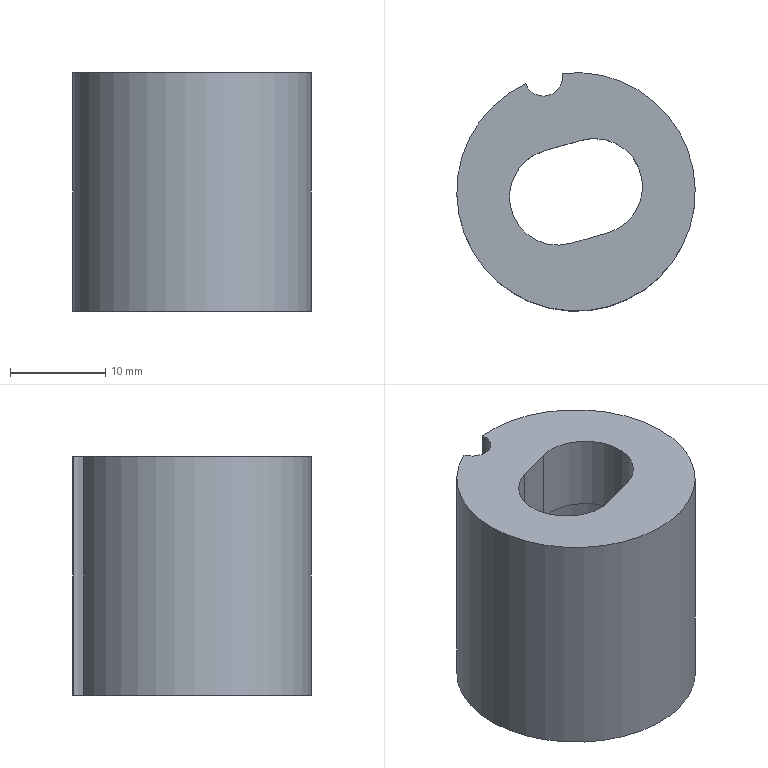Part | NX | features solid 2 | 1 solid | 10 faces | box 25 x 25 x 25 mm | volume 7477 mm3 | cylinder 5 | plane 5 | commonest cylinder face diameters 10.1 x2 4 x1 16.6 x1 25 x1
STEP:
#1=CARTESIAN_POINT('',(529.721,-368.981,-7.));
#2=VERTEX_POINT('',#1);
#3=CARTESIAN_POINT('',(529.721,-368.981,18.));
#4=VERTEX_POINT('',#3);
#5=CARTESIAN_POINT('',(529.721,-368.981,5.5));
#6=DIRECTION('',(0.,0.,1.));
#7=VECTOR('',#6,1000.);
#8=LINE('',#5,#7);
#9=EDGE_CURVE('',#2,#4,#8,.T.);
#10=ORIENTED_EDGE('',*,*,#9,.F.);
#11=CARTESIAN_POINT('',(533.558,-367.895,-7.));
#12=VERTEX_POINT('',#11);
#13=CARTESIAN_POINT('',(535.,-380.311,-7.));
#14=DIRECTION('',(0.,0.,1.));
#15=DIRECTION('',(-0.2723,0.9622,0.));
#16=AXIS2_PLACEMENT_3D('',#13,#14,#15);
#17=CIRCLE('',#16,12.5);
#18=EDGE_CURVE('',#2,#12,#17,.T.);
#19=ORIENTED_EDGE('',*,*,#18,.T.);
#20=CARTESIAN_POINT('',(533.558,-367.895,18.));
#21=VERTEX_POINT('',#20);
#22=CARTESIAN_POINT('',(533.558,-367.895,5.5));
#23=DIRECTION('',(0.,0.,1.));
#24=VECTOR('',#23,1000.);
#25=LINE('',#22,#24);
#26=EDGE_CURVE('',#21,#12,#25,.F.);
#27=ORIENTED_EDGE('',*,*,#26,.F.);
#28=CARTESIAN_POINT('',(535.,-380.311,18.));
#29=DIRECTION('',(0.,0.,1.));
#30=DIRECTION('',(-0.2723,0.9622,0.));
#31=AXIS2_PLACEMENT_3D('',#28,#29,#30);
#32=CIRCLE('',#31,12.5);
#33=EDGE_CURVE('',#4,#21,#32,.T.);
#34=ORIENTED_EDGE('',*,*,#33,.F.);
#35=EDGE_LOOP('',(#10,#19,#27,#34));
#36=FACE_BOUND('',#35,.T.);
#37=CARTESIAN_POINT('',(535.,-380.311,-7.));
#38=DIRECTION('',(0.,0.,1.));
#39=DIRECTION('',(-0.2723,0.9622,0.));
#40=AXIS2_PLACEMENT_3D('',#37,#38,#39);
#41=CYLINDRICAL_SURFACE('',#40,12.5);
#42=ADVANCED_FACE('',(#36),#41,.T.);
#43=CARTESIAN_POINT('',(532.74,-372.325,-7.));
#44=VERTEX_POINT('',#43);
#45=CARTESIAN_POINT('',(535.,-380.311,-7.));
#46=DIRECTION('',(0.,0.,1.));
#47=DIRECTION('',(-0.2723,0.9622,0.));
#48=AXIS2_PLACEMENT_3D('',#45,#46,#47);
#49=CIRCLE('',#48,8.3);
#50=EDGE_CURVE('',#44,#44,#49,.T.);
#51=ORIENTED_EDGE('',*,*,#50,.T.);
#52=EDGE_LOOP('',(#51));
#53=FACE_BOUND('',#52,.T.);
#54=ORIENTED_EDGE('',*,*,#18,.F.);
#55=CARTESIAN_POINT('',(531.596,-368.284,-7.));
#56=DIRECTION('',(0.,0.,1.));
#57=DIRECTION('',(-0.2723,0.9622,0.));
#58=AXIS2_PLACEMENT_3D('',#55,#56,#57);
#59=CIRCLE('',#58,2.);
#60=EDGE_CURVE('',#2,#12,#59,.T.);
#61=ORIENTED_EDGE('',*,*,#60,.T.);
#62=EDGE_LOOP('',(#54,#61));
#63=FACE_BOUND('',#62,.T.);
#64=CARTESIAN_POINT('',(535.,-380.311,-7.));
#65=DIRECTION('',(0.,0.,1.));
#66=DIRECTION('',(-0.2723,0.9622,0.));
#67=AXIS2_PLACEMENT_3D('',#64,#65,#66);
#68=PLANE('',#67);
#69=ADVANCED_FACE('',(#53,#63),#68,.F.);
#70=CARTESIAN_POINT('',(534.451,-385.715,18.));
#71=VERTEX_POINT('',#70);
#72=CARTESIAN_POINT('',(538.3,-384.626,18.));
#73=VERTEX_POINT('',#72);
#74=CARTESIAN_POINT('',(534.451,-385.715,18.));
#75=DIRECTION('',(0.9622,0.2723,0.));
#76=VECTOR('',#75,1000.);
#77=LINE('',#74,#76);
#78=EDGE_CURVE('',#71,#73,#77,.T.);
#79=ORIENTED_EDGE('',*,*,#78,.F.);
#80=CARTESIAN_POINT('',(531.7,-375.997,18.));
#81=VERTEX_POINT('',#80);
#82=CARTESIAN_POINT('',(533.076,-380.856,18.));
#83=DIRECTION('',(0.,0.,1.));
#84=DIRECTION('',(-0.2723,0.9622,0.));
#85=AXIS2_PLACEMENT_3D('',#82,#83,#84);
#86=CIRCLE('',#85,5.05);
#87=EDGE_CURVE('',#81,#71,#86,.T.);
#88=ORIENTED_EDGE('',*,*,#87,.F.);
#89=CARTESIAN_POINT('',(535.549,-374.908,18.));
#90=VERTEX_POINT('',#89);
#91=CARTESIAN_POINT('',(531.7,-375.997,18.));
#92=DIRECTION('',(0.9622,0.2723,0.));
#93=VECTOR('',#92,1000.);
#94=LINE('',#91,#93);
#95=EDGE_CURVE('',#81,#90,#94,.T.);
#96=ORIENTED_EDGE('',*,*,#95,.T.);
#97=CARTESIAN_POINT('',(536.924,-379.767,18.));
#98=DIRECTION('',(0.,0.,1.));
#99=DIRECTION('',(-0.2723,0.9622,0.));
#100=AXIS2_PLACEMENT_3D('',#97,#98,#99);
#101=CIRCLE('',#100,5.05);
#102=EDGE_CURVE('',#73,#90,#101,.T.);
#103=ORIENTED_EDGE('',*,*,#102,.F.);
#104=EDGE_LOOP('',(#79,#88,#96,#103));
#105=FACE_BOUND('',#104,.T.);
#106=CARTESIAN_POINT('',(531.596,-368.284,18.));
#107=DIRECTION('',(0.,0.,1.));
#108=DIRECTION('',(-0.2723,0.9622,0.));
#109=AXIS2_PLACEMENT_3D('',#106,#107,#108);
#110=CIRCLE('',#109,2.);
#111=EDGE_CURVE('',#4,#21,#110,.T.);
#112=ORIENTED_EDGE('',*,*,#111,.F.);
#113=ORIENTED_EDGE('',*,*,#33,.T.);
#114=EDGE_LOOP('',(#112,#113));
#115=FACE_BOUND('',#114,.T.);
#116=CARTESIAN_POINT('',(535.,-380.311,18.));
#117=DIRECTION('',(0.,0.,1.));
#118=DIRECTION('',(-0.2723,0.9622,0.));
#119=AXIS2_PLACEMENT_3D('',#116,#117,#118);
#120=PLANE('',#119);
#121=ADVANCED_FACE('',(#105,#115),#120,.T.);
#122=ORIENTED_EDGE('',*,*,#50,.F.);
#123=EDGE_LOOP('',(#122));
#124=FACE_BOUND('',#123,.T.);
#125=CARTESIAN_POINT('',(532.74,-372.325,10.));
#126=VERTEX_POINT('',#125);
#127=CARTESIAN_POINT('',(535.,-380.311,10.));
#128=DIRECTION('',(0.,0.,1.));
#129=DIRECTION('',(-0.2723,0.9622,0.));
#130=AXIS2_PLACEMENT_3D('',#127,#128,#129);
#131=CIRCLE('',#130,8.3);
#132=EDGE_CURVE('',#126,#126,#131,.T.);
#133=ORIENTED_EDGE('',*,*,#132,.T.);
#134=EDGE_LOOP('',(#133));
#135=FACE_BOUND('',#134,.T.);
#136=CARTESIAN_POINT('',(535.,-380.311,-7.));
#137=DIRECTION('',(0.,0.,1.));
#138=DIRECTION('',(-0.2723,0.9622,0.));
#139=AXIS2_PLACEMENT_3D('',#136,#137,#138);
#140=CYLINDRICAL_SURFACE('',#139,8.3);
#141=ADVANCED_FACE('',(#124,#135),#140,.F.);
#142=CARTESIAN_POINT('',(531.7,-375.997,10.));
#143=VERTEX_POINT('',#142);
#144=CARTESIAN_POINT('',(534.451,-385.715,10.));
#145=VERTEX_POINT('',#144);
#146=CARTESIAN_POINT('',(533.076,-380.856,10.));
#147=DIRECTION('',(0.,0.,1.));
#148=DIRECTION('',(-0.2723,0.9622,0.));
#149=AXIS2_PLACEMENT_3D('',#146,#147,#148);
#150=CIRCLE('',#149,5.05);
#151=EDGE_CURVE('',#143,#145,#150,.T.);
#152=ORIENTED_EDGE('',*,*,#151,.T.);
#153=CARTESIAN_POINT('',(538.3,-384.626,10.));
#154=VERTEX_POINT('',#153);
#155=CARTESIAN_POINT('',(536.375,-385.171,10.));
#156=DIRECTION('',(0.9622,0.2723,0.));
#157=VECTOR('',#156,1000.);
#158=LINE('',#155,#157);
#159=EDGE_CURVE('',#145,#154,#158,.T.);
#160=ORIENTED_EDGE('',*,*,#159,.T.);
#161=CARTESIAN_POINT('',(535.549,-374.908,10.));
#162=VERTEX_POINT('',#161);
#163=CARTESIAN_POINT('',(536.924,-379.767,10.));
#164=DIRECTION('',(0.,0.,1.));
#165=DIRECTION('',(-0.2723,0.9622,0.));
#166=AXIS2_PLACEMENT_3D('',#163,#164,#165);
#167=CIRCLE('',#166,5.05);
#168=EDGE_CURVE('',#154,#162,#167,.T.);
#169=ORIENTED_EDGE('',*,*,#168,.T.);
#170=CARTESIAN_POINT('',(533.625,-375.452,10.));
#171=DIRECTION('',(0.9622,0.2723,0.));
#172=VECTOR('',#171,1000.);
#173=LINE('',#170,#172);
#174=EDGE_CURVE('',#143,#162,#173,.T.);
#175=ORIENTED_EDGE('',*,*,#174,.F.);
#176=EDGE_LOOP('',(#152,#160,#169,#175));
#177=FACE_BOUND('',#176,.T.);
#178=ORIENTED_EDGE('',*,*,#132,.F.);
#179=EDGE_LOOP('',(#178));
#180=FACE_BOUND('',#179,.T.);
#181=CARTESIAN_POINT('',(535.,-380.311,10.));
#182=DIRECTION('',(0.,0.,1.));
#183=DIRECTION('',(-0.2723,0.9622,0.));
#184=AXIS2_PLACEMENT_3D('',#181,#182,#183);
#185=PLANE('',#184);
#186=ADVANCED_FACE('',(#177,#180),#185,.F.);
#187=ORIENTED_EDGE('',*,*,#9,.T.);
#188=ORIENTED_EDGE('',*,*,#111,.T.);
#189=ORIENTED_EDGE('',*,*,#26,.T.);
#190=ORIENTED_EDGE('',*,*,#60,.F.);
#191=EDGE_LOOP('',(#187,#188,#189,#190));
#192=FACE_BOUND('',#191,.T.);
#193=CARTESIAN_POINT('',(531.596,-368.284,-7.));
#194=DIRECTION('',(0.,0.,1.));
#195=DIRECTION('',(-0.2723,0.9622,0.));
#196=AXIS2_PLACEMENT_3D('',#193,#194,#195);
#197=CYLINDRICAL_SURFACE('',#196,2.);
#198=ADVANCED_FACE('',(#192),#197,.F.);
#199=CARTESIAN_POINT('',(534.451,-385.715,-7.));
#200=DIRECTION('',(0.,0.,1.));
#201=VECTOR('',#200,1000.);
#202=LINE('',#199,#201);
#203=EDGE_CURVE('',#145,#71,#202,.T.);
#204=ORIENTED_EDGE('',*,*,#203,.T.);
#205=ORIENTED_EDGE('',*,*,#78,.T.);
#206=CARTESIAN_POINT('',(538.3,-384.626,-7.));
#207=DIRECTION('',(0.,0.,1.));
#208=VECTOR('',#207,1000.);
#209=LINE('',#206,#208);
#210=EDGE_CURVE('',#154,#73,#209,.T.);
#211=ORIENTED_EDGE('',*,*,#210,.F.);
#212=ORIENTED_EDGE('',*,*,#159,.F.);
#213=EDGE_LOOP('',(#204,#205,#211,#212));
#214=FACE_BOUND('',#213,.T.);
#215=CARTESIAN_POINT('',(534.451,-385.715,-7.));
#216=DIRECTION('',(0.2723,-0.9622,0.));
#217=DIRECTION('',(0.,0.,1.));
#218=AXIS2_PLACEMENT_3D('',#215,#216,#217);
#219=PLANE('',#218);
#220=ADVANCED_FACE('',(#214),#219,.F.);
#221=ORIENTED_EDGE('',*,*,#210,.T.);
#222=ORIENTED_EDGE('',*,*,#102,.T.);
#223=CARTESIAN_POINT('',(535.549,-374.908,-7.));
#224=DIRECTION('',(0.,0.,1.));
#225=VECTOR('',#224,1000.);
#226=LINE('',#223,#225);
#227=EDGE_CURVE('',#162,#90,#226,.T.);
#228=ORIENTED_EDGE('',*,*,#227,.F.);
#229=ORIENTED_EDGE('',*,*,#168,.F.);
#230=EDGE_LOOP('',(#221,#222,#228,#229));
#231=FACE_BOUND('',#230,.T.);
#232=CARTESIAN_POINT('',(536.924,-379.767,-7.));
#233=DIRECTION('',(0.,0.,1.));
#234=DIRECTION('',(-0.2723,0.9622,0.));
#235=AXIS2_PLACEMENT_3D('',#232,#233,#234);
#236=CYLINDRICAL_SURFACE('',#235,5.05);
#237=ADVANCED_FACE('',(#231),#236,.F.);
#238=ORIENTED_EDGE('',*,*,#174,.T.);
#239=ORIENTED_EDGE('',*,*,#227,.T.);
#240=ORIENTED_EDGE('',*,*,#95,.F.);
#241=CARTESIAN_POINT('',(531.7,-375.997,-7.));
#242=DIRECTION('',(0.,0.,1.));
#243=VECTOR('',#242,1000.);
#244=LINE('',#241,#243);
#245=EDGE_CURVE('',#143,#81,#244,.T.);
#246=ORIENTED_EDGE('',*,*,#245,.F.);
#247=EDGE_LOOP('',(#238,#239,#240,#246));
#248=FACE_BOUND('',#247,.T.);
#249=CARTESIAN_POINT('',(531.7,-375.997,-7.));
#250=DIRECTION('',(0.2723,-0.9622,0.));
#251=DIRECTION('',(0.,0.,1.));
#252=AXIS2_PLACEMENT_3D('',#249,#250,#251);
#253=PLANE('',#252);
#254=ADVANCED_FACE('',(#248),#253,.T.);
#255=ORIENTED_EDGE('',*,*,#245,.T.);
#256=ORIENTED_EDGE('',*,*,#87,.T.);
#257=ORIENTED_EDGE('',*,*,#203,.F.);
#258=ORIENTED_EDGE('',*,*,#151,.F.);
#259=EDGE_LOOP('',(#255,#256,#257,#258));
#260=FACE_BOUND('',#259,.T.);
#261=CARTESIAN_POINT('',(533.076,-380.856,-7.));
#262=DIRECTION('',(0.,0.,1.));
#263=DIRECTION('',(-0.2723,0.9622,0.));
#264=AXIS2_PLACEMENT_3D('',#261,#262,#263);
#265=CYLINDRICAL_SURFACE('',#264,5.05);
#266=ADVANCED_FACE('',(#260),#265,.F.);
#267=CLOSED_SHELL('',(#42,#69,#121,#141,#186,#198,#220,#237,#254,#266));
#268=MANIFOLD_SOLID_BREP('',#267);
#269=(LENGTH_UNIT()NAMED_UNIT(*)SI_UNIT(.MILLI.,.METRE.));
#270=UNCERTAINTY_MEASURE_WITH_UNIT(LENGTH_MEASURE(0.00001),#269,'','');
#271=(NAMED_UNIT(*)PLANE_ANGLE_UNIT()SI_UNIT($,.RADIAN.));
#272=(NAMED_UNIT(*)SI_UNIT($,.STERADIAN.)SOLID_ANGLE_UNIT());
#273=(GEOMETRIC_REPRESENTATION_CONTEXT(3)GLOBAL_UNCERTAINTY_ASSIGNED_CONTEXT((#270))GLOBAL_UNIT_ASSIGNED_CONTEXT((#269,#271,#272))REPRESENTATION_CONTEXT('',''));
#274=ADVANCED_BREP_SHAPE_REPRESENTATION('',(#268),#273);